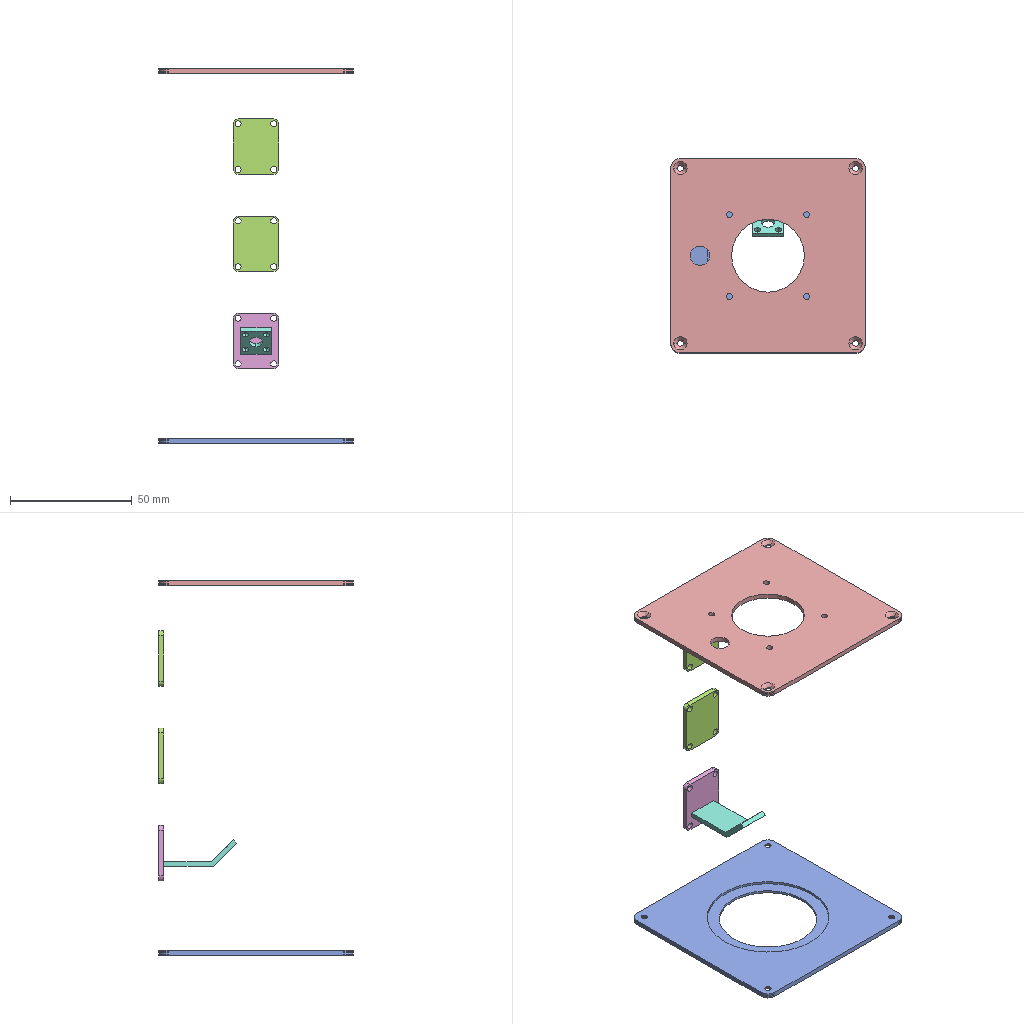Assembly | SolidWorks | 11 different items | 12 placed | box 80 x 80 x 154 mm
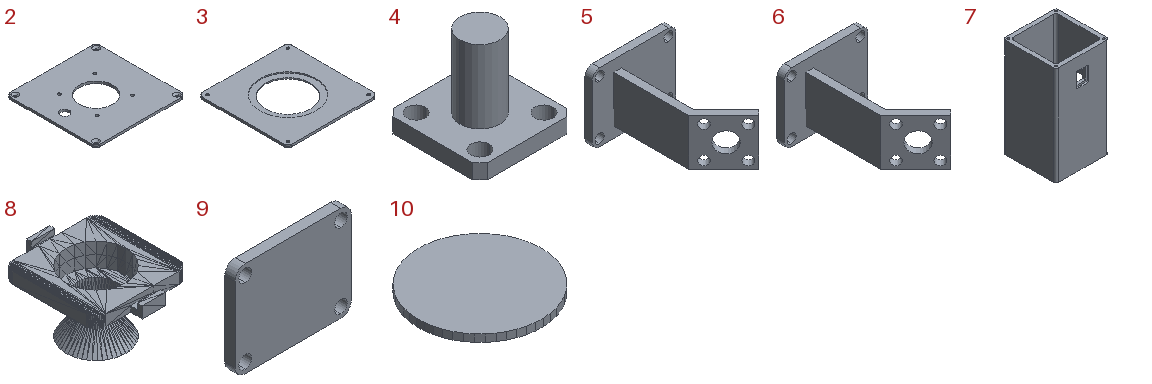Parts list (item | name | quantity | size | volume | features):
1 | - | x1 | - | - | -
2 | - | x1 | 80 x 80 x 2 mm | 11130 mm3 | features ICE 4, Chamfer 1, Extrusion 1, MoveFace 1
3 | - | x1 | 80 x 80 x 2 mm | 9472 mm3 | features ICE 7, Chamfer 1, Extrusion 1, MoveFace 1
4 | - | x1 | 12.7 x 12.7 x 11.8 mm | 503.752 mm3 | features ICE 2, Chamfer 1, Extrusion 1
5 | - | x1 | 22.8 x 32.073 x 18.7 mm | 1563 mm3 | features ICE 4, ExtruThin 1, Fillet 1
6 | - | x1 | 22.8 x 32.073 x 18.7 mm | 1563 mm3 | features ICE 4, ExtruThin 1, Fillet 1
7 | - | x1 | 80 x 80 x 150 mm | 261015 mm3 | features ICE 7, Fillet 3, Extrusion 1, MirrorPattern 1
8 | - | x1 | - | - | features RefSurface 4
9 | - | x2 | 22.8 x 2 x 18.7 mm | 806.583 mm3 | features ICE 5, ExtruThin 1, Fillet 1
10 | - | x1 | 49.972 x 49.978 x 3 mm | 5875 mm3 | features Extrusion 1
11 | Housing2 | x1 | - | - | -
Mates (type | each side: item.copy, entity, surface, feature):
DistanceDim | 3.1 face plane Boss-Extrude1 | 2.1 face plane Boss-Extrude1
Width | 2.1 face plane Boss-Extrude1 | 2.1 face plane Boss-Extrude1 | 3.1 face plane Boss-Extrude1 | 3.1 face plane Boss-Extrude1 | 2 times